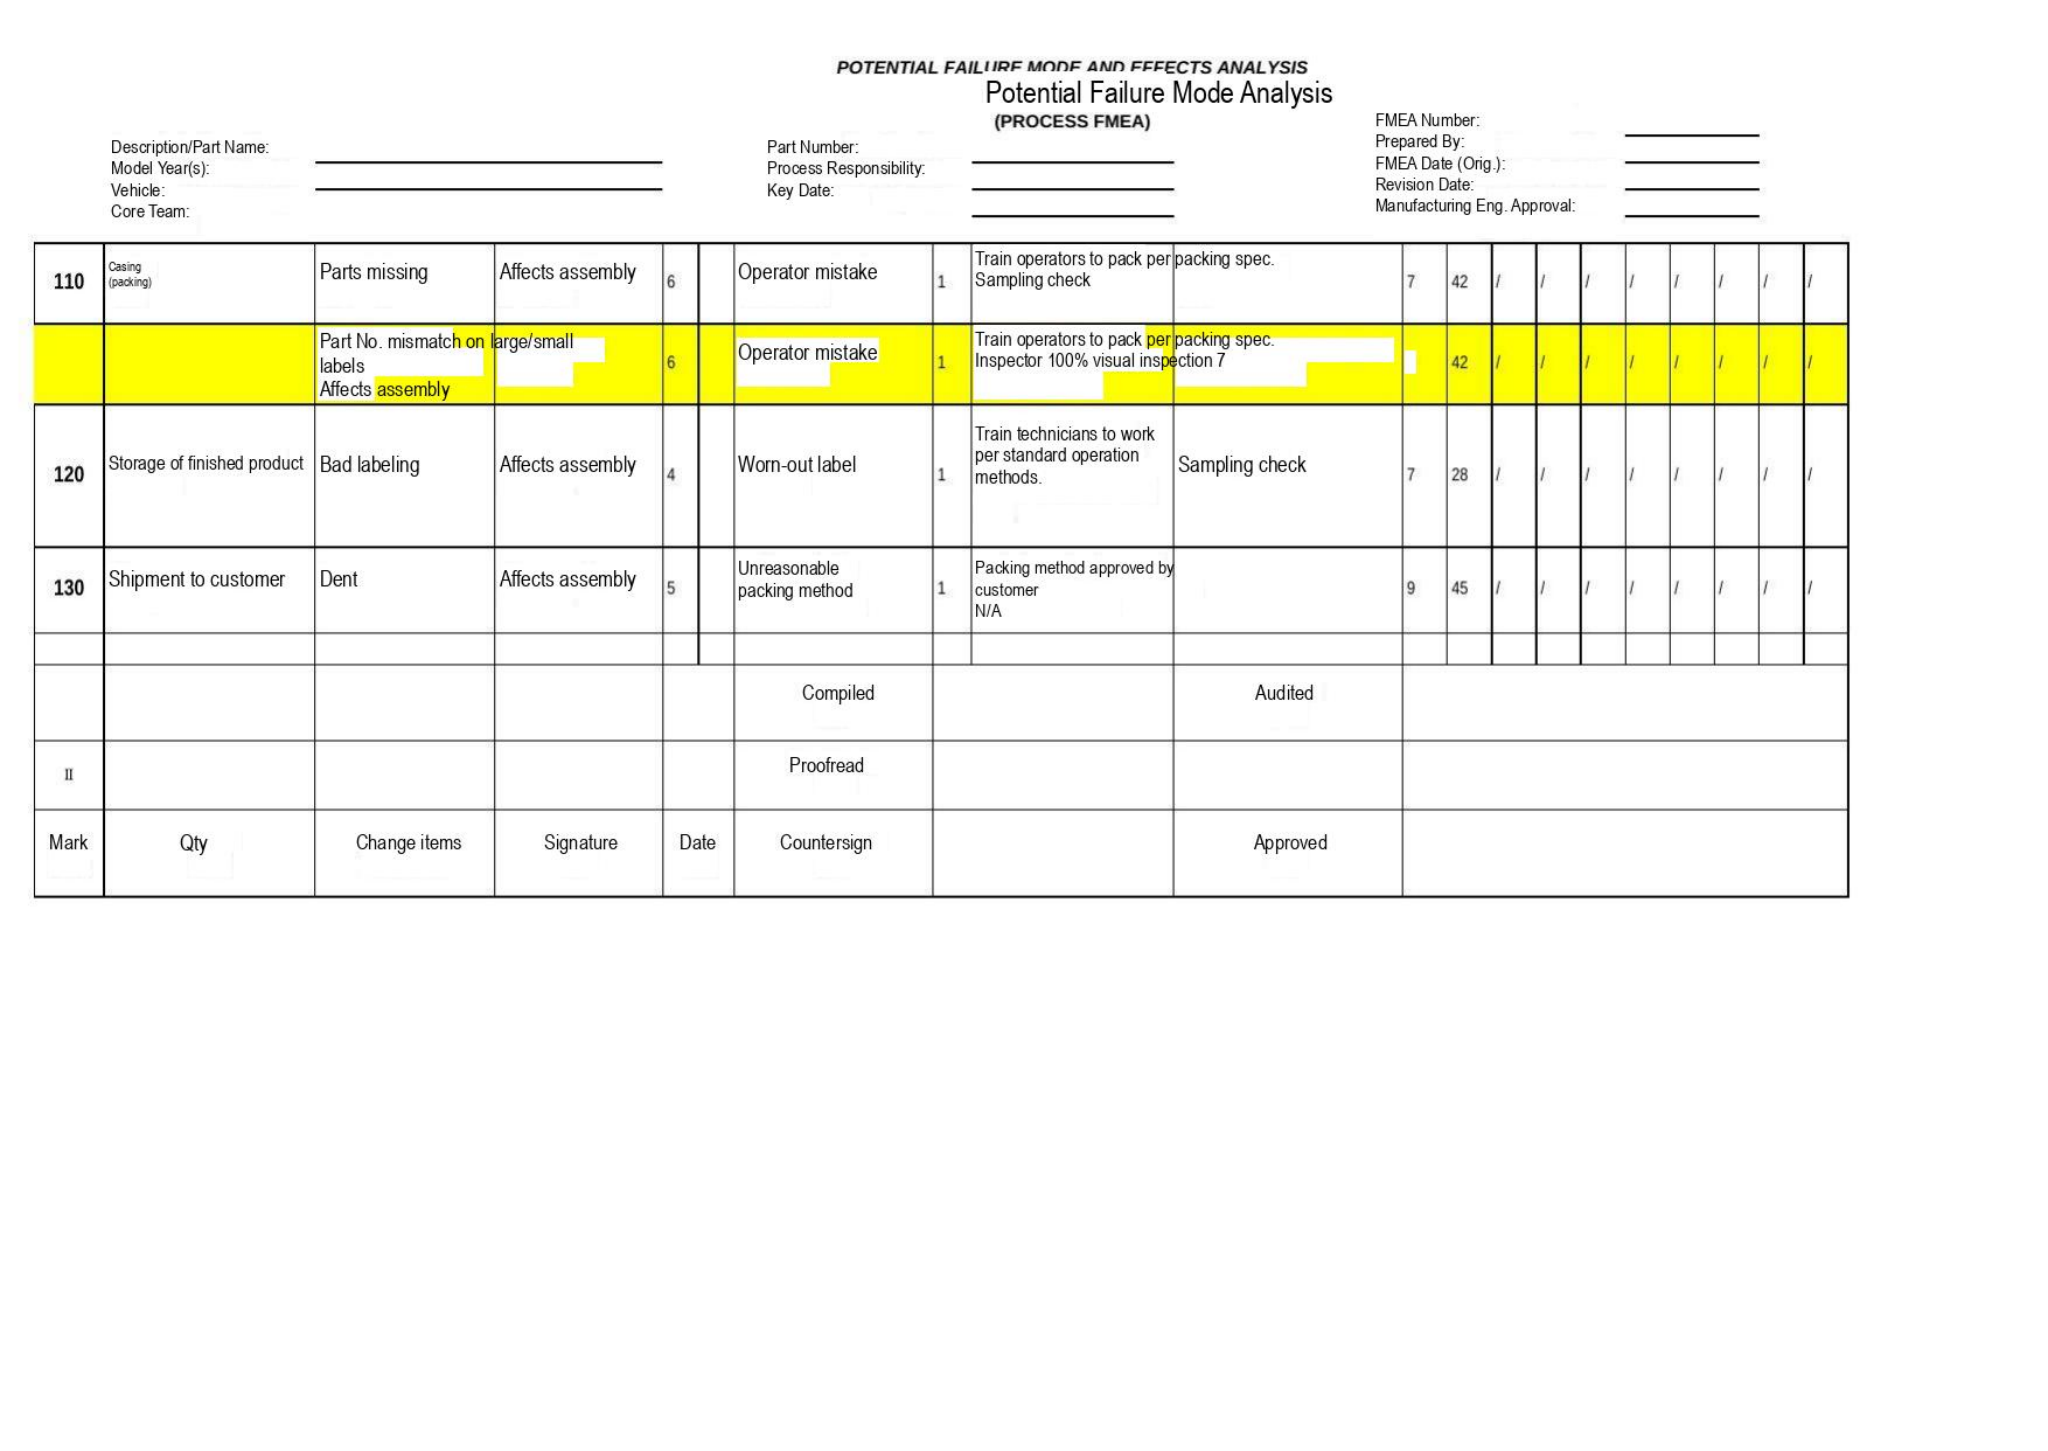POTENTIAL FAILURE MODE AND EFFECTS ANALYSIS
Potential Failure Mode Analysis
(PROCESS FMEA)

Description/Part Name:
Model Year(s):
Vehicle:
Core Team:

Part Number:
Process Responsibility:
Key Date:

FMEA Number:
Prepared By:
FMEA Date (Orig.):
Revision Date:
Manufacturing Eng. Approval:

| | | | | | | | | | | | | | | | | | | | |
|---|---|---|---|---|---|---|---|---|---|---|---|---|---|---|---|---|---|---|---|
| 110 | Casing (packing) | Parts missing | Affects assembly | 6 | | Operator mistake | 1 | Train operators to pack per packing spec.<br>Sampling check | | 7 | 42 | / | / | / | / | / | / | / | / |
| | | Part No. mismatch on large/small labels<br>Affects assembly | | 6 | | Operator mistake | 1 | Train operators to pack per packing spec.<br>Inspector 100% visual inspection 7 | | | 42 | / | / | / | / | / | / | / | / |
| 120 | Storage of finished product | Bad labeling | Affects assembly | 4 | | Worn-out label | 1 | Train technicians to work per standard operation methods. | Sampling check | 7 | 28 | / | / | / | / | / | / | / | / |
| 130 | Shipment to customer | Dent | Affects assembly | 5 | | Unreasonable packing method | 1 | Packing method approved by customer<br>N/A | | 9 | 45 | / | / | / | / | / | / | / | / |
| | | | | | | | | | | | | | | | | | | | |

| | | | | | | | | |
|---|---|---|---|---|---|---|---|---|
| | | | | | Compiled | | Audited | |
| II | | | | | Proofread | | | |
| Mark | Qty | Change items | Signature | Date | Countersign | | Approved | |